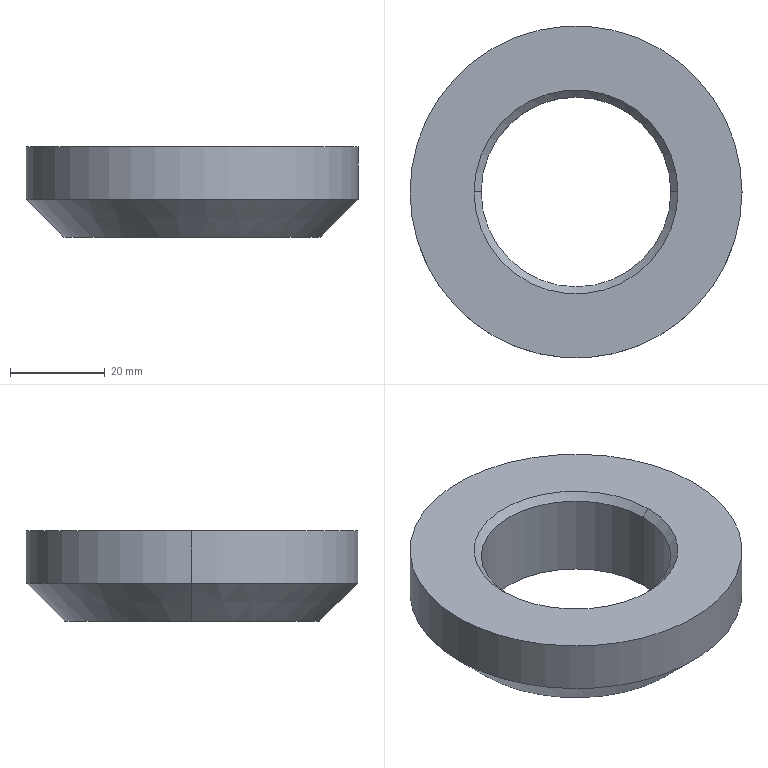Part | SolidWorks | features Chamfer 2, Extrusion 1 | 1 solid | 10 faces | box 70 x 70 x 19 mm | volume 42599 mm3 | cone 4 | cylinder 4 | plane 2 | commonest cylinder face diameters 40 x2 70 x2
STEP:
#1=CARTESIAN_POINT('',(-20.,0.,17.5));
#2=VERTEX_POINT('',#1);
#3=CARTESIAN_POINT('',(20.,0.,17.5));
#4=VERTEX_POINT('',#3);
#5=CARTESIAN_POINT('',(0.,0.,17.5));
#6=DIRECTION('',(0.,0.,1.));
#7=DIRECTION('',(1.,0.,0.));
#8=AXIS2_PLACEMENT_3D('',#5,#6,#7);
#9=CIRCLE('',#8,20.);
#10=EDGE_CURVE('',#2,#4,#9,.T.);
#11=ORIENTED_EDGE('',*,*,#10,.F.);
#12=CARTESIAN_POINT('',(-21.5,0.,19.));
#13=VERTEX_POINT('',#12);
#14=CARTESIAN_POINT('',(-20.,0.,17.5));
#15=DIRECTION('',(-0.7071,0.,0.7071));
#16=VECTOR('',#15,1000.);
#17=LINE('',#14,#16);
#18=EDGE_CURVE('',#2,#13,#17,.T.);
#19=ORIENTED_EDGE('',*,*,#18,.T.);
#20=CARTESIAN_POINT('',(21.5,0.,19.));
#21=VERTEX_POINT('',#20);
#22=CARTESIAN_POINT('',(0.,0.,19.));
#23=DIRECTION('',(0.,0.,-1.));
#24=DIRECTION('',(1.,0.,0.));
#25=AXIS2_PLACEMENT_3D('',#22,#23,#24);
#26=CIRCLE('',#25,21.5);
#27=EDGE_CURVE('',#21,#13,#26,.T.);
#28=ORIENTED_EDGE('',*,*,#27,.F.);
#29=CARTESIAN_POINT('',(20.,0.,17.5));
#30=DIRECTION('',(0.7071,0.,0.7071));
#31=VECTOR('',#30,1000.);
#32=LINE('',#29,#31);
#33=EDGE_CURVE('',#4,#21,#32,.T.);
#34=ORIENTED_EDGE('',*,*,#33,.F.);
#35=EDGE_LOOP('',(#11,#19,#28,#34));
#36=FACE_OUTER_BOUND('',#35,.T.);
#37=CARTESIAN_POINT('',(0.,0.,17.5));
#38=DIRECTION('',(0.,0.,1.));
#39=DIRECTION('',(1.,0.,0.));
#40=AXIS2_PLACEMENT_3D('',#37,#38,#39);
#41=CONICAL_SURFACE('',#40,20.,0.7854);
#42=ADVANCED_FACE('',(#36),#41,.F.);
#43=CARTESIAN_POINT('',(-27.,0.,0.));
#44=VERTEX_POINT('',#43);
#45=CARTESIAN_POINT('',(27.,0.,0.));
#46=VERTEX_POINT('',#45);
#47=CARTESIAN_POINT('',(0.,0.,0.));
#48=DIRECTION('',(0.,0.,-1.));
#49=DIRECTION('',(1.,0.,0.));
#50=AXIS2_PLACEMENT_3D('',#47,#48,#49);
#51=CIRCLE('',#50,27.);
#52=EDGE_CURVE('',#44,#46,#51,.T.);
#53=ORIENTED_EDGE('',*,*,#52,.F.);
#54=CARTESIAN_POINT('',(-35.,0.,8.));
#55=VERTEX_POINT('',#54);
#56=CARTESIAN_POINT('',(-35.,0.,8.));
#57=DIRECTION('',(-0.7071,0.,0.7071));
#58=VECTOR('',#57,1000.);
#59=LINE('',#56,#58);
#60=EDGE_CURVE('',#44,#55,#59,.T.);
#61=ORIENTED_EDGE('',*,*,#60,.T.);
#62=CARTESIAN_POINT('',(35.,0.,8.));
#63=VERTEX_POINT('',#62);
#64=CARTESIAN_POINT('',(0.,0.,8.));
#65=DIRECTION('',(0.,0.,1.));
#66=DIRECTION('',(1.,0.,0.));
#67=AXIS2_PLACEMENT_3D('',#64,#65,#66);
#68=CIRCLE('',#67,35.);
#69=EDGE_CURVE('',#63,#55,#68,.T.);
#70=ORIENTED_EDGE('',*,*,#69,.F.);
#71=CARTESIAN_POINT('',(35.,0.,8.));
#72=DIRECTION('',(0.7071,0.,0.7071));
#73=VECTOR('',#72,1000.);
#74=LINE('',#71,#73);
#75=EDGE_CURVE('',#46,#63,#74,.T.);
#76=ORIENTED_EDGE('',*,*,#75,.F.);
#77=EDGE_LOOP('',(#53,#61,#70,#76));
#78=FACE_OUTER_BOUND('',#77,.T.);
#79=CARTESIAN_POINT('',(0.,0.,8.));
#80=DIRECTION('',(0.,0.,1.));
#81=DIRECTION('',(1.,0.,0.));
#82=AXIS2_PLACEMENT_3D('',#79,#80,#81);
#83=CONICAL_SURFACE('',#82,35.,0.7854);
#84=ADVANCED_FACE('',(#78),#83,.T.);
#85=ORIENTED_EDGE('',*,*,#10,.T.);
#86=CARTESIAN_POINT('',(20.,0.,0.));
#87=VERTEX_POINT('',#86);
#88=CARTESIAN_POINT('',(20.,0.,19.));
#89=DIRECTION('',(0.,0.,-1.));
#90=VECTOR('',#89,1000.);
#91=LINE('',#88,#90);
#92=EDGE_CURVE('',#4,#87,#91,.T.);
#93=ORIENTED_EDGE('',*,*,#92,.T.);
#94=CARTESIAN_POINT('',(-20.,0.,0.));
#95=VERTEX_POINT('',#94);
#96=CARTESIAN_POINT('',(0.,0.,0.));
#97=DIRECTION('',(0.,0.,1.));
#98=DIRECTION('',(1.,0.,0.));
#99=AXIS2_PLACEMENT_3D('',#96,#97,#98);
#100=CIRCLE('',#99,20.);
#101=EDGE_CURVE('',#95,#87,#100,.T.);
#102=ORIENTED_EDGE('',*,*,#101,.F.);
#103=CARTESIAN_POINT('',(-20.,0.,19.));
#104=DIRECTION('',(0.,0.,-1.));
#105=VECTOR('',#104,1000.);
#106=LINE('',#103,#105);
#107=EDGE_CURVE('',#2,#95,#106,.T.);
#108=ORIENTED_EDGE('',*,*,#107,.F.);
#109=EDGE_LOOP('',(#85,#93,#102,#108));
#110=FACE_OUTER_BOUND('',#109,.T.);
#111=CARTESIAN_POINT('',(0.,0.,19.));
#112=DIRECTION('',(0.,0.,-1.));
#113=DIRECTION('',(-1.,0.,0.));
#114=AXIS2_PLACEMENT_3D('',#111,#112,#113);
#115=CYLINDRICAL_SURFACE('',#114,20.);
#116=ADVANCED_FACE('',(#110),#115,.F.);
#117=CARTESIAN_POINT('',(35.,0.,19.));
#118=VERTEX_POINT('',#117);
#119=CARTESIAN_POINT('',(-35.,0.,19.));
#120=VERTEX_POINT('',#119);
#121=CARTESIAN_POINT('',(0.,0.,19.));
#122=DIRECTION('',(0.,0.,1.));
#123=DIRECTION('',(1.,0.,0.));
#124=AXIS2_PLACEMENT_3D('',#121,#122,#123);
#125=CIRCLE('',#124,35.);
#126=EDGE_CURVE('',#118,#120,#125,.T.);
#127=ORIENTED_EDGE('',*,*,#126,.F.);
#128=CARTESIAN_POINT('',(35.,0.,19.));
#129=DIRECTION('',(0.,0.,-1.));
#130=VECTOR('',#129,1000.);
#131=LINE('',#128,#130);
#132=EDGE_CURVE('',#118,#63,#131,.T.);
#133=ORIENTED_EDGE('',*,*,#132,.T.);
#134=ORIENTED_EDGE('',*,*,#69,.T.);
#135=CARTESIAN_POINT('',(-35.,0.,19.));
#136=DIRECTION('',(0.,0.,-1.));
#137=VECTOR('',#136,1000.);
#138=LINE('',#135,#137);
#139=EDGE_CURVE('',#120,#55,#138,.T.);
#140=ORIENTED_EDGE('',*,*,#139,.F.);
#141=EDGE_LOOP('',(#127,#133,#134,#140));
#142=FACE_OUTER_BOUND('',#141,.T.);
#143=CARTESIAN_POINT('',(0.,0.,19.));
#144=DIRECTION('',(0.,0.,-1.));
#145=DIRECTION('',(-1.,0.,0.));
#146=AXIS2_PLACEMENT_3D('',#143,#144,#145);
#147=CYLINDRICAL_SURFACE('',#146,35.);
#148=ADVANCED_FACE('',(#142),#147,.T.);
#149=ORIENTED_EDGE('',*,*,#27,.T.);
#150=CARTESIAN_POINT('',(0.,0.,19.));
#151=DIRECTION('',(0.,0.,-1.));
#152=DIRECTION('',(1.,0.,0.));
#153=AXIS2_PLACEMENT_3D('',#150,#151,#152);
#154=CIRCLE('',#153,21.5);
#155=EDGE_CURVE('',#13,#21,#154,.T.);
#156=ORIENTED_EDGE('',*,*,#155,.T.);
#157=EDGE_LOOP('',(#149,#156));
#158=FACE_BOUND('',#157,.T.);
#159=CARTESIAN_POINT('',(0.,0.,19.));
#160=DIRECTION('',(0.,0.,1.));
#161=DIRECTION('',(1.,0.,0.));
#162=AXIS2_PLACEMENT_3D('',#159,#160,#161);
#163=CIRCLE('',#162,35.);
#164=EDGE_CURVE('',#120,#118,#163,.T.);
#165=ORIENTED_EDGE('',*,*,#164,.T.);
#166=ORIENTED_EDGE('',*,*,#126,.T.);
#167=EDGE_LOOP('',(#165,#166));
#168=FACE_OUTER_BOUND('',#167,.T.);
#169=CARTESIAN_POINT('',(0.,0.,19.));
#170=DIRECTION('',(0.,0.,1.));
#171=DIRECTION('',(1.,0.,0.));
#172=AXIS2_PLACEMENT_3D('',#169,#170,#171);
#173=PLANE('',#172);
#174=ADVANCED_FACE('',(#158,#168),#173,.T.);
#175=CARTESIAN_POINT('',(0.,0.,0.));
#176=DIRECTION('',(0.,0.,-1.));
#177=DIRECTION('',(1.,0.,0.));
#178=AXIS2_PLACEMENT_3D('',#175,#176,#177);
#179=CIRCLE('',#178,27.);
#180=EDGE_CURVE('',#46,#44,#179,.T.);
#181=ORIENTED_EDGE('',*,*,#180,.T.);
#182=ORIENTED_EDGE('',*,*,#52,.T.);
#183=EDGE_LOOP('',(#181,#182));
#184=FACE_OUTER_BOUND('',#183,.T.);
#185=ORIENTED_EDGE('',*,*,#101,.T.);
#186=CARTESIAN_POINT('',(0.,0.,0.));
#187=DIRECTION('',(0.,0.,1.));
#188=DIRECTION('',(1.,0.,0.));
#189=AXIS2_PLACEMENT_3D('',#186,#187,#188);
#190=CIRCLE('',#189,20.);
#191=EDGE_CURVE('',#87,#95,#190,.T.);
#192=ORIENTED_EDGE('',*,*,#191,.T.);
#193=EDGE_LOOP('',(#185,#192));
#194=FACE_BOUND('',#193,.T.);
#195=CARTESIAN_POINT('',(0.,0.,0.));
#196=DIRECTION('',(0.,0.,1.));
#197=DIRECTION('',(1.,0.,0.));
#198=AXIS2_PLACEMENT_3D('',#195,#196,#197);
#199=PLANE('',#198);
#200=ADVANCED_FACE('',(#184,#194),#199,.F.);
#201=ORIENTED_EDGE('',*,*,#132,.F.);
#202=ORIENTED_EDGE('',*,*,#164,.F.);
#203=ORIENTED_EDGE('',*,*,#139,.T.);
#204=CARTESIAN_POINT('',(0.,0.,8.));
#205=DIRECTION('',(0.,0.,1.));
#206=DIRECTION('',(1.,0.,0.));
#207=AXIS2_PLACEMENT_3D('',#204,#205,#206);
#208=CIRCLE('',#207,35.);
#209=EDGE_CURVE('',#55,#63,#208,.T.);
#210=ORIENTED_EDGE('',*,*,#209,.T.);
#211=EDGE_LOOP('',(#201,#202,#203,#210));
#212=FACE_OUTER_BOUND('',#211,.T.);
#213=CARTESIAN_POINT('',(0.,0.,19.));
#214=DIRECTION('',(0.,0.,-1.));
#215=DIRECTION('',(-1.,0.,0.));
#216=AXIS2_PLACEMENT_3D('',#213,#214,#215);
#217=CYLINDRICAL_SURFACE('',#216,35.);
#218=ADVANCED_FACE('',(#212),#217,.T.);
#219=ORIENTED_EDGE('',*,*,#92,.F.);
#220=CARTESIAN_POINT('',(0.,0.,17.5));
#221=DIRECTION('',(0.,0.,1.));
#222=DIRECTION('',(1.,0.,0.));
#223=AXIS2_PLACEMENT_3D('',#220,#221,#222);
#224=CIRCLE('',#223,20.);
#225=EDGE_CURVE('',#4,#2,#224,.T.);
#226=ORIENTED_EDGE('',*,*,#225,.T.);
#227=ORIENTED_EDGE('',*,*,#107,.T.);
#228=ORIENTED_EDGE('',*,*,#191,.F.);
#229=EDGE_LOOP('',(#219,#226,#227,#228));
#230=FACE_OUTER_BOUND('',#229,.T.);
#231=CARTESIAN_POINT('',(0.,0.,19.));
#232=DIRECTION('',(0.,0.,-1.));
#233=DIRECTION('',(-1.,0.,0.));
#234=AXIS2_PLACEMENT_3D('',#231,#232,#233);
#235=CYLINDRICAL_SURFACE('',#234,20.);
#236=ADVANCED_FACE('',(#230),#235,.F.);
#237=ORIENTED_EDGE('',*,*,#60,.F.);
#238=ORIENTED_EDGE('',*,*,#180,.F.);
#239=ORIENTED_EDGE('',*,*,#75,.T.);
#240=ORIENTED_EDGE('',*,*,#209,.F.);
#241=EDGE_LOOP('',(#237,#238,#239,#240));
#242=FACE_OUTER_BOUND('',#241,.T.);
#243=CARTESIAN_POINT('',(0.,0.,8.));
#244=DIRECTION('',(0.,0.,1.));
#245=DIRECTION('',(1.,0.,0.));
#246=AXIS2_PLACEMENT_3D('',#243,#244,#245);
#247=CONICAL_SURFACE('',#246,35.,0.7854);
#248=ADVANCED_FACE('',(#242),#247,.T.);
#249=ORIENTED_EDGE('',*,*,#18,.F.);
#250=ORIENTED_EDGE('',*,*,#225,.F.);
#251=ORIENTED_EDGE('',*,*,#33,.T.);
#252=ORIENTED_EDGE('',*,*,#155,.F.);
#253=EDGE_LOOP('',(#249,#250,#251,#252));
#254=FACE_OUTER_BOUND('',#253,.T.);
#255=CARTESIAN_POINT('',(0.,0.,17.5));
#256=DIRECTION('',(0.,0.,1.));
#257=DIRECTION('',(1.,0.,0.));
#258=AXIS2_PLACEMENT_3D('',#255,#256,#257);
#259=CONICAL_SURFACE('',#258,20.,0.7854);
#260=ADVANCED_FACE('',(#254),#259,.F.);
#261=CLOSED_SHELL('',(#42,#84,#116,#148,#174,#200,#218,#236,#248,#260));
#262=MANIFOLD_SOLID_BREP('',#261);
#263=CARTESIAN_POINT('',(0.,0.,0.));
#264=DIRECTION('',(0.,0.,1.));
#265=DIRECTION('',(1.,0.,0.));
#266=AXIS2_PLACEMENT_3D('',#263,#264,#265);
#267=(LENGTH_UNIT()NAMED_UNIT(*)SI_UNIT(.MILLI.,.METRE.));
#268=UNCERTAINTY_MEASURE_WITH_UNIT(LENGTH_MEASURE(0.00001),#267,'','');
#269=(NAMED_UNIT(*)PLANE_ANGLE_UNIT()SI_UNIT($,.RADIAN.));
#270=(NAMED_UNIT(*)SI_UNIT($,.STERADIAN.)SOLID_ANGLE_UNIT());
#271=(GEOMETRIC_REPRESENTATION_CONTEXT(3)GLOBAL_UNCERTAINTY_ASSIGNED_CONTEXT((#268))GLOBAL_UNIT_ASSIGNED_CONTEXT((#267,#269,#270))REPRESENTATION_CONTEXT('',''));
#272=ADVANCED_BREP_SHAPE_REPRESENTATION('',(#262,#266),#271);